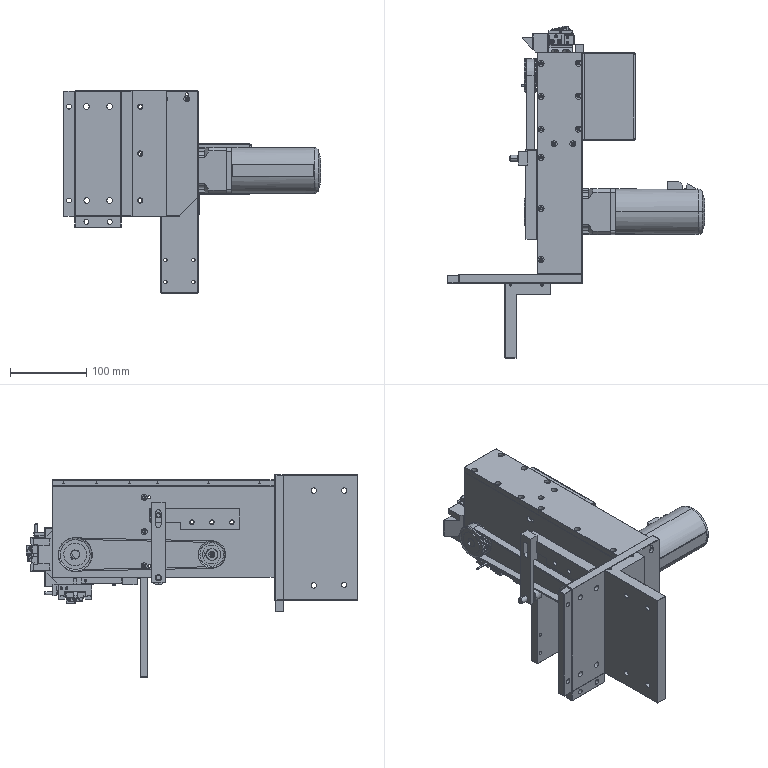Part | NX | 90 solids | 4456 faces | volume 2481997 mm3 | plane 1936 | cylinder 1698 | cone 662 | torus 112 | sphere 44 | spline 4 | commonest cylinder face diameters 2.5 x244 3.3 x238 6.55 x97 0.5 x96 1.1 x93 4.5 x77